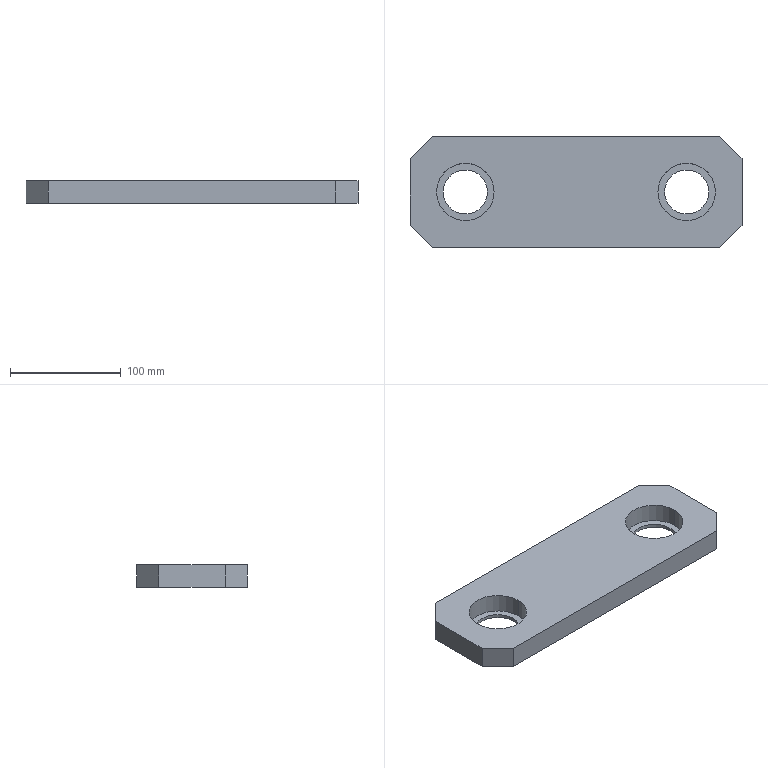Part | SolidWorks | features BaseBody 1 | 1 solid | 20 faces | box 300 x 100 x 20 mm | volume 504254 mm3 | plane 12 | cylinder 8 | commonest cylinder face diameters 40 x4 52 x4
STEP:
#1=CARTESIAN_POINT('',(198.047,1592.079,-399.));
#2=VERTEX_POINT('',#1);
#3=CARTESIAN_POINT('',(158.047,1592.079,-399.));
#4=VERTEX_POINT('',#3);
#5=CARTESIAN_POINT('',(178.047,1592.079,-399.));
#6=DIRECTION('',(0.,0.,-1.));
#7=DIRECTION('',(1.,0.,0.));
#8=AXIS2_PLACEMENT_3D('',#5,#6,#7);
#9=CIRCLE('',#8,20.);
#10=EDGE_CURVE('',#2,#4,#9,.T.);
#11=ORIENTED_EDGE('',*,*,#10,.T.);
#12=CARTESIAN_POINT('',(158.047,1592.079,-396.));
#13=VERTEX_POINT('',#12);
#14=CARTESIAN_POINT('',(158.047,1592.079,-455.569));
#15=DIRECTION('',(0.,0.,1.));
#16=VECTOR('',#15,1000.);
#17=LINE('',#14,#16);
#18=EDGE_CURVE('',#4,#13,#17,.T.);
#19=ORIENTED_EDGE('',*,*,#18,.T.);
#20=CARTESIAN_POINT('',(198.047,1592.079,-396.));
#21=VERTEX_POINT('',#20);
#22=CARTESIAN_POINT('',(178.047,1592.079,-396.));
#23=DIRECTION('',(0.,0.,-1.));
#24=DIRECTION('',(1.,0.,0.));
#25=AXIS2_PLACEMENT_3D('',#22,#23,#24);
#26=CIRCLE('',#25,20.);
#27=EDGE_CURVE('',#21,#13,#26,.T.);
#28=ORIENTED_EDGE('',*,*,#27,.F.);
#29=CARTESIAN_POINT('',(198.047,1592.079,-455.569));
#30=DIRECTION('',(0.,0.,1.));
#31=VECTOR('',#30,1000.);
#32=LINE('',#29,#31);
#33=EDGE_CURVE('',#2,#21,#32,.T.);
#34=ORIENTED_EDGE('',*,*,#33,.F.);
#35=EDGE_LOOP('',(#11,#19,#28,#34));
#36=FACE_OUTER_BOUND('',#35,.T.);
#37=CARTESIAN_POINT('',(178.047,1592.079,-455.569));
#38=DIRECTION('',(0.,0.,1.));
#39=DIRECTION('',(1.,0.,0.));
#40=AXIS2_PLACEMENT_3D('',#37,#38,#39);
#41=CYLINDRICAL_SURFACE('',#40,20.);
#42=ADVANCED_FACE('',(#36),#41,.F.);
#43=CARTESIAN_POINT('',(-1.953,1592.079,-399.));
#44=VERTEX_POINT('',#43);
#45=CARTESIAN_POINT('',(-41.953,1592.079,-399.));
#46=VERTEX_POINT('',#45);
#47=CARTESIAN_POINT('',(-21.953,1592.079,-399.));
#48=DIRECTION('',(0.,0.,-1.));
#49=DIRECTION('',(1.,0.,0.));
#50=AXIS2_PLACEMENT_3D('',#47,#48,#49);
#51=CIRCLE('',#50,20.);
#52=EDGE_CURVE('',#44,#46,#51,.T.);
#53=ORIENTED_EDGE('',*,*,#52,.T.);
#54=CARTESIAN_POINT('',(-41.953,1592.079,-396.));
#55=VERTEX_POINT('',#54);
#56=CARTESIAN_POINT('',(-41.953,1592.079,-455.569));
#57=DIRECTION('',(0.,0.,1.));
#58=VECTOR('',#57,1000.);
#59=LINE('',#56,#58);
#60=EDGE_CURVE('',#46,#55,#59,.T.);
#61=ORIENTED_EDGE('',*,*,#60,.T.);
#62=CARTESIAN_POINT('',(-1.953,1592.079,-396.));
#63=VERTEX_POINT('',#62);
#64=CARTESIAN_POINT('',(-21.953,1592.079,-396.));
#65=DIRECTION('',(0.,0.,-1.));
#66=DIRECTION('',(1.,0.,0.));
#67=AXIS2_PLACEMENT_3D('',#64,#65,#66);
#68=CIRCLE('',#67,20.);
#69=EDGE_CURVE('',#63,#55,#68,.T.);
#70=ORIENTED_EDGE('',*,*,#69,.F.);
#71=CARTESIAN_POINT('',(-1.953,1592.079,-455.569));
#72=DIRECTION('',(0.,0.,1.));
#73=VECTOR('',#72,1000.);
#74=LINE('',#71,#73);
#75=EDGE_CURVE('',#44,#63,#74,.T.);
#76=ORIENTED_EDGE('',*,*,#75,.F.);
#77=EDGE_LOOP('',(#53,#61,#70,#76));
#78=FACE_OUTER_BOUND('',#77,.T.);
#79=CARTESIAN_POINT('',(-21.953,1592.079,-455.569));
#80=DIRECTION('',(0.,0.,1.));
#81=DIRECTION('',(1.,0.,0.));
#82=AXIS2_PLACEMENT_3D('',#79,#80,#81);
#83=CYLINDRICAL_SURFACE('',#82,20.);
#84=ADVANCED_FACE('',(#78),#83,.F.);
#85=CARTESIAN_POINT('',(204.047,1592.079,-396.));
#86=VERTEX_POINT('',#85);
#87=CARTESIAN_POINT('',(152.047,1592.079,-396.));
#88=VERTEX_POINT('',#87);
#89=CARTESIAN_POINT('',(178.047,1592.079,-396.));
#90=DIRECTION('',(0.,0.,-1.));
#91=DIRECTION('',(1.,0.,0.));
#92=AXIS2_PLACEMENT_3D('',#89,#90,#91);
#93=CIRCLE('',#92,26.);
#94=EDGE_CURVE('',#86,#88,#93,.T.);
#95=ORIENTED_EDGE('',*,*,#94,.T.);
#96=CARTESIAN_POINT('',(152.047,1592.079,-379.));
#97=VERTEX_POINT('',#96);
#98=CARTESIAN_POINT('',(152.047,1592.079,-396.));
#99=DIRECTION('',(0.,0.,1.));
#100=VECTOR('',#99,1000.);
#101=LINE('',#98,#100);
#102=EDGE_CURVE('',#88,#97,#101,.T.);
#103=ORIENTED_EDGE('',*,*,#102,.T.);
#104=CARTESIAN_POINT('',(204.047,1592.079,-379.));
#105=VERTEX_POINT('',#104);
#106=CARTESIAN_POINT('',(178.047,1592.079,-379.));
#107=DIRECTION('',(0.,0.,-1.));
#108=DIRECTION('',(1.,0.,0.));
#109=AXIS2_PLACEMENT_3D('',#106,#107,#108);
#110=CIRCLE('',#109,26.);
#111=EDGE_CURVE('',#105,#97,#110,.T.);
#112=ORIENTED_EDGE('',*,*,#111,.F.);
#113=CARTESIAN_POINT('',(204.047,1592.079,-396.));
#114=DIRECTION('',(0.,0.,1.));
#115=VECTOR('',#114,1000.);
#116=LINE('',#113,#115);
#117=EDGE_CURVE('',#86,#105,#116,.T.);
#118=ORIENTED_EDGE('',*,*,#117,.F.);
#119=EDGE_LOOP('',(#95,#103,#112,#118));
#120=FACE_OUTER_BOUND('',#119,.T.);
#121=CARTESIAN_POINT('',(178.047,1592.079,-396.));
#122=DIRECTION('',(0.,0.,1.));
#123=DIRECTION('',(1.,0.,0.));
#124=AXIS2_PLACEMENT_3D('',#121,#122,#123);
#125=CYLINDRICAL_SURFACE('',#124,26.);
#126=ADVANCED_FACE('',(#120),#125,.F.);
#127=CARTESIAN_POINT('',(-47.953,1592.079,-396.));
#128=VERTEX_POINT('',#127);
#129=CARTESIAN_POINT('',(4.047,1592.079,-396.));
#130=VERTEX_POINT('',#129);
#131=CARTESIAN_POINT('',(-21.953,1592.079,-396.));
#132=DIRECTION('',(0.,0.,1.));
#133=DIRECTION('',(1.,0.,0.));
#134=AXIS2_PLACEMENT_3D('',#131,#132,#133);
#135=CIRCLE('',#134,26.);
#136=EDGE_CURVE('',#128,#130,#135,.T.);
#137=ORIENTED_EDGE('',*,*,#136,.F.);
#138=CARTESIAN_POINT('',(-47.953,1592.079,-379.));
#139=VERTEX_POINT('',#138);
#140=CARTESIAN_POINT('',(-47.953,1592.079,-396.));
#141=DIRECTION('',(0.,0.,1.));
#142=VECTOR('',#141,1000.);
#143=LINE('',#140,#142);
#144=EDGE_CURVE('',#128,#139,#143,.T.);
#145=ORIENTED_EDGE('',*,*,#144,.T.);
#146=CARTESIAN_POINT('',(4.047,1592.079,-379.));
#147=VERTEX_POINT('',#146);
#148=CARTESIAN_POINT('',(-21.953,1592.079,-379.));
#149=DIRECTION('',(0.,0.,-1.));
#150=DIRECTION('',(1.,0.,0.));
#151=AXIS2_PLACEMENT_3D('',#148,#149,#150);
#152=CIRCLE('',#151,26.);
#153=EDGE_CURVE('',#147,#139,#152,.T.);
#154=ORIENTED_EDGE('',*,*,#153,.F.);
#155=CARTESIAN_POINT('',(4.047,1592.079,-396.));
#156=DIRECTION('',(0.,0.,1.));
#157=VECTOR('',#156,1000.);
#158=LINE('',#155,#157);
#159=EDGE_CURVE('',#130,#147,#158,.T.);
#160=ORIENTED_EDGE('',*,*,#159,.F.);
#161=EDGE_LOOP('',(#137,#145,#154,#160));
#162=FACE_OUTER_BOUND('',#161,.T.);
#163=CARTESIAN_POINT('',(-21.953,1592.079,-396.));
#164=DIRECTION('',(0.,0.,1.));
#165=DIRECTION('',(1.,0.,0.));
#166=AXIS2_PLACEMENT_3D('',#163,#164,#165);
#167=CYLINDRICAL_SURFACE('',#166,26.);
#168=ADVANCED_FACE('',(#162),#167,.F.);
#169=ORIENTED_EDGE('',*,*,#10,.F.);
#170=CARTESIAN_POINT('',(178.047,1592.079,-399.));
#171=DIRECTION('',(0.,0.,-1.));
#172=DIRECTION('',(1.,0.,0.));
#173=AXIS2_PLACEMENT_3D('',#170,#171,#172);
#174=CIRCLE('',#173,20.);
#175=EDGE_CURVE('',#4,#2,#174,.T.);
#176=ORIENTED_EDGE('',*,*,#175,.F.);
#177=EDGE_LOOP('',(#169,#176));
#178=FACE_BOUND('',#177,.T.);
#179=ORIENTED_EDGE('',*,*,#52,.F.);
#180=CARTESIAN_POINT('',(-21.953,1592.079,-399.));
#181=DIRECTION('',(0.,0.,-1.));
#182=DIRECTION('',(1.,0.,0.));
#183=AXIS2_PLACEMENT_3D('',#180,#181,#182);
#184=CIRCLE('',#183,20.);
#185=EDGE_CURVE('',#46,#44,#184,.T.);
#186=ORIENTED_EDGE('',*,*,#185,.F.);
#187=EDGE_LOOP('',(#179,#186));
#188=FACE_BOUND('',#187,.T.);
#189=CARTESIAN_POINT('',(228.047,1562.079,-399.));
#190=VERTEX_POINT('',#189);
#191=CARTESIAN_POINT('',(228.047,1622.079,-399.));
#192=VERTEX_POINT('',#191);
#193=CARTESIAN_POINT('',(228.047,1542.079,-399.));
#194=DIRECTION('',(0.,1.,0.));
#195=VECTOR('',#194,1000.);
#196=LINE('',#193,#195);
#197=EDGE_CURVE('',#190,#192,#196,.T.);
#198=ORIENTED_EDGE('',*,*,#197,.F.);
#199=CARTESIAN_POINT('',(208.047,1542.079,-399.));
#200=VERTEX_POINT('',#199);
#201=CARTESIAN_POINT('',(208.047,1542.079,-399.));
#202=DIRECTION('',(0.7071,0.7071,0.));
#203=VECTOR('',#202,1000.);
#204=LINE('',#201,#203);
#205=EDGE_CURVE('',#200,#190,#204,.T.);
#206=ORIENTED_EDGE('',*,*,#205,.F.);
#207=CARTESIAN_POINT('',(-51.953,1542.079,-399.));
#208=VERTEX_POINT('',#207);
#209=CARTESIAN_POINT('',(-71.953,1542.079,-399.));
#210=DIRECTION('',(1.,0.,0.));
#211=VECTOR('',#210,1000.);
#212=LINE('',#209,#211);
#213=EDGE_CURVE('',#208,#200,#212,.T.);
#214=ORIENTED_EDGE('',*,*,#213,.F.);
#215=CARTESIAN_POINT('',(-71.953,1562.079,-399.));
#216=VERTEX_POINT('',#215);
#217=CARTESIAN_POINT('',(-71.953,1562.079,-399.));
#218=DIRECTION('',(0.7071,-0.7071,0.));
#219=VECTOR('',#218,1000.);
#220=LINE('',#217,#219);
#221=EDGE_CURVE('',#216,#208,#220,.T.);
#222=ORIENTED_EDGE('',*,*,#221,.F.);
#223=CARTESIAN_POINT('',(-71.953,1622.079,-399.));
#224=VERTEX_POINT('',#223);
#225=CARTESIAN_POINT('',(-71.953,1542.079,-399.));
#226=DIRECTION('',(0.,-1.,0.));
#227=VECTOR('',#226,1000.);
#228=LINE('',#225,#227);
#229=EDGE_CURVE('',#224,#216,#228,.T.);
#230=ORIENTED_EDGE('',*,*,#229,.F.);
#231=CARTESIAN_POINT('',(-51.953,1642.079,-399.));
#232=VERTEX_POINT('',#231);
#233=CARTESIAN_POINT('',(-51.953,1642.079,-399.));
#234=DIRECTION('',(-0.7071,-0.7071,0.));
#235=VECTOR('',#234,1000.);
#236=LINE('',#233,#235);
#237=EDGE_CURVE('',#232,#224,#236,.T.);
#238=ORIENTED_EDGE('',*,*,#237,.F.);
#239=CARTESIAN_POINT('',(208.047,1642.079,-399.));
#240=VERTEX_POINT('',#239);
#241=CARTESIAN_POINT('',(-71.953,1642.079,-399.));
#242=DIRECTION('',(-1.,0.,0.));
#243=VECTOR('',#242,1000.);
#244=LINE('',#241,#243);
#245=EDGE_CURVE('',#240,#232,#244,.T.);
#246=ORIENTED_EDGE('',*,*,#245,.F.);
#247=CARTESIAN_POINT('',(228.047,1622.079,-399.));
#248=DIRECTION('',(-0.7071,0.7071,0.));
#249=VECTOR('',#248,1000.);
#250=LINE('',#247,#249);
#251=EDGE_CURVE('',#192,#240,#250,.T.);
#252=ORIENTED_EDGE('',*,*,#251,.F.);
#253=EDGE_LOOP('',(#198,#206,#214,#222,#230,#238,#246,#252));
#254=FACE_OUTER_BOUND('',#253,.T.);
#255=CARTESIAN_POINT('',(-71.953,1542.079,-399.));
#256=DIRECTION('',(0.,0.,1.));
#257=DIRECTION('',(1.,0.,0.));
#258=AXIS2_PLACEMENT_3D('',#255,#256,#257);
#259=PLANE('',#258);
#260=ADVANCED_FACE('',(#178,#188,#254),#259,.F.);
#261=ORIENTED_EDGE('',*,*,#18,.F.);
#262=ORIENTED_EDGE('',*,*,#175,.T.);
#263=ORIENTED_EDGE('',*,*,#33,.T.);
#264=CARTESIAN_POINT('',(178.047,1592.079,-396.));
#265=DIRECTION('',(0.,0.,-1.));
#266=DIRECTION('',(1.,0.,0.));
#267=AXIS2_PLACEMENT_3D('',#264,#265,#266);
#268=CIRCLE('',#267,20.);
#269=EDGE_CURVE('',#13,#21,#268,.T.);
#270=ORIENTED_EDGE('',*,*,#269,.F.);
#271=EDGE_LOOP('',(#261,#262,#263,#270));
#272=FACE_OUTER_BOUND('',#271,.T.);
#273=CARTESIAN_POINT('',(178.047,1592.079,-455.569));
#274=DIRECTION('',(0.,0.,1.));
#275=DIRECTION('',(1.,0.,0.));
#276=AXIS2_PLACEMENT_3D('',#273,#274,#275);
#277=CYLINDRICAL_SURFACE('',#276,20.);
#278=ADVANCED_FACE('',(#272),#277,.F.);
#279=ORIENTED_EDGE('',*,*,#60,.F.);
#280=ORIENTED_EDGE('',*,*,#185,.T.);
#281=ORIENTED_EDGE('',*,*,#75,.T.);
#282=CARTESIAN_POINT('',(-21.953,1592.079,-396.));
#283=DIRECTION('',(0.,0.,-1.));
#284=DIRECTION('',(1.,0.,0.));
#285=AXIS2_PLACEMENT_3D('',#282,#283,#284);
#286=CIRCLE('',#285,20.);
#287=EDGE_CURVE('',#55,#63,#286,.T.);
#288=ORIENTED_EDGE('',*,*,#287,.F.);
#289=EDGE_LOOP('',(#279,#280,#281,#288));
#290=FACE_OUTER_BOUND('',#289,.T.);
#291=CARTESIAN_POINT('',(-21.953,1592.079,-455.569));
#292=DIRECTION('',(0.,0.,1.));
#293=DIRECTION('',(1.,0.,0.));
#294=AXIS2_PLACEMENT_3D('',#291,#292,#293);
#295=CYLINDRICAL_SURFACE('',#294,20.);
#296=ADVANCED_FACE('',(#290),#295,.F.);
#297=ORIENTED_EDGE('',*,*,#251,.T.);
#298=CARTESIAN_POINT('',(208.047,1642.079,-379.));
#299=VERTEX_POINT('',#298);
#300=CARTESIAN_POINT('',(208.047,1642.079,-379.));
#301=DIRECTION('',(0.,0.,-1.));
#302=VECTOR('',#301,1000.);
#303=LINE('',#300,#302);
#304=EDGE_CURVE('',#299,#240,#303,.T.);
#305=ORIENTED_EDGE('',*,*,#304,.F.);
#306=CARTESIAN_POINT('',(228.047,1622.079,-379.));
#307=VERTEX_POINT('',#306);
#308=CARTESIAN_POINT('',(208.047,1642.079,-379.));
#309=DIRECTION('',(-0.7071,0.7071,0.));
#310=VECTOR('',#309,1000.);
#311=LINE('',#308,#310);
#312=EDGE_CURVE('',#307,#299,#311,.T.);
#313=ORIENTED_EDGE('',*,*,#312,.F.);
#314=CARTESIAN_POINT('',(228.047,1622.079,-379.));
#315=DIRECTION('',(0.,0.,1.));
#316=VECTOR('',#315,1000.);
#317=LINE('',#314,#316);
#318=EDGE_CURVE('',#192,#307,#317,.T.);
#319=ORIENTED_EDGE('',*,*,#318,.F.);
#320=EDGE_LOOP('',(#297,#305,#313,#319));
#321=FACE_OUTER_BOUND('',#320,.T.);
#322=CARTESIAN_POINT('',(208.047,1642.079,-379.));
#323=DIRECTION('',(-0.7071,-0.7071,0.));
#324=DIRECTION('',(0.7071,-0.7071,0.));
#325=AXIS2_PLACEMENT_3D('',#322,#323,#324);
#326=PLANE('',#325);
#327=ADVANCED_FACE('',(#321),#326,.F.);
#328=CARTESIAN_POINT('',(228.047,1562.079,-379.));
#329=VERTEX_POINT('',#328);
#330=CARTESIAN_POINT('',(228.047,1642.079,-379.));
#331=DIRECTION('',(0.,1.,0.));
#332=VECTOR('',#331,1000.);
#333=LINE('',#330,#332);
#334=EDGE_CURVE('',#329,#307,#333,.T.);
#335=ORIENTED_EDGE('',*,*,#334,.F.);
#336=CARTESIAN_POINT('',(228.047,1562.079,-379.));
#337=DIRECTION('',(0.,0.,1.));
#338=VECTOR('',#337,1000.);
#339=LINE('',#336,#338);
#340=EDGE_CURVE('',#190,#329,#339,.T.);
#341=ORIENTED_EDGE('',*,*,#340,.F.);
#342=ORIENTED_EDGE('',*,*,#197,.T.);
#343=ORIENTED_EDGE('',*,*,#318,.T.);
#344=EDGE_LOOP('',(#335,#341,#342,#343));
#345=FACE_OUTER_BOUND('',#344,.T.);
#346=CARTESIAN_POINT('',(228.047,1642.079,-379.));
#347=DIRECTION('',(-1.,0.,0.));
#348=DIRECTION('',(0.,0.,1.));
#349=AXIS2_PLACEMENT_3D('',#346,#347,#348);
#350=PLANE('',#349);
#351=ADVANCED_FACE('',(#345),#350,.F.);
#352=ORIENTED_EDGE('',*,*,#205,.T.);
#353=ORIENTED_EDGE('',*,*,#340,.T.);
#354=CARTESIAN_POINT('',(208.047,1542.079,-379.));
#355=VERTEX_POINT('',#354);
#356=CARTESIAN_POINT('',(228.047,1562.079,-379.));
#357=DIRECTION('',(0.7071,0.7071,0.));
#358=VECTOR('',#357,1000.);
#359=LINE('',#356,#358);
#360=EDGE_CURVE('',#355,#329,#359,.T.);
#361=ORIENTED_EDGE('',*,*,#360,.F.);
#362=CARTESIAN_POINT('',(208.047,1542.079,-379.));
#363=DIRECTION('',(0.,0.,1.));
#364=VECTOR('',#363,1000.);
#365=LINE('',#362,#364);
#366=EDGE_CURVE('',#200,#355,#365,.T.);
#367=ORIENTED_EDGE('',*,*,#366,.F.);
#368=EDGE_LOOP('',(#352,#353,#361,#367));
#369=FACE_OUTER_BOUND('',#368,.T.);
#370=CARTESIAN_POINT('',(228.047,1562.079,-379.));
#371=DIRECTION('',(-0.7071,0.7071,0.));
#372=DIRECTION('',(-0.7071,-0.7071,0.));
#373=AXIS2_PLACEMENT_3D('',#370,#371,#372);
#374=PLANE('',#373);
#375=ADVANCED_FACE('',(#369),#374,.F.);
#376=CARTESIAN_POINT('',(-51.953,1542.079,-379.));
#377=VERTEX_POINT('',#376);
#378=CARTESIAN_POINT('',(-71.953,1542.079,-379.));
#379=DIRECTION('',(1.,0.,0.));
#380=VECTOR('',#379,1000.);
#381=LINE('',#378,#380);
#382=EDGE_CURVE('',#377,#355,#381,.T.);
#383=ORIENTED_EDGE('',*,*,#382,.F.);
#384=CARTESIAN_POINT('',(-51.953,1542.079,-379.));
#385=DIRECTION('',(0.,0.,1.));
#386=VECTOR('',#385,1000.);
#387=LINE('',#384,#386);
#388=EDGE_CURVE('',#208,#377,#387,.T.);
#389=ORIENTED_EDGE('',*,*,#388,.F.);
#390=ORIENTED_EDGE('',*,*,#213,.T.);
#391=ORIENTED_EDGE('',*,*,#366,.T.);
#392=EDGE_LOOP('',(#383,#389,#390,#391));
#393=FACE_OUTER_BOUND('',#392,.T.);
#394=CARTESIAN_POINT('',(-71.953,1542.079,-379.));
#395=DIRECTION('',(0.,1.,0.));
#396=DIRECTION('',(0.,0.,1.));
#397=AXIS2_PLACEMENT_3D('',#394,#395,#396);
#398=PLANE('',#397);
#399=ADVANCED_FACE('',(#393),#398,.F.);
#400=ORIENTED_EDGE('',*,*,#221,.T.);
#401=ORIENTED_EDGE('',*,*,#388,.T.);
#402=CARTESIAN_POINT('',(-71.953,1562.079,-379.));
#403=VERTEX_POINT('',#402);
#404=CARTESIAN_POINT('',(-51.953,1542.079,-379.));
#405=DIRECTION('',(0.7071,-0.7071,0.));
#406=VECTOR('',#405,1000.);
#407=LINE('',#404,#406);
#408=EDGE_CURVE('',#403,#377,#407,.T.);
#409=ORIENTED_EDGE('',*,*,#408,.F.);
#410=CARTESIAN_POINT('',(-71.953,1562.079,-379.));
#411=DIRECTION('',(0.,0.,1.));
#412=VECTOR('',#411,1000.);
#413=LINE('',#410,#412);
#414=EDGE_CURVE('',#216,#403,#413,.T.);
#415=ORIENTED_EDGE('',*,*,#414,.F.);
#416=EDGE_LOOP('',(#400,#401,#409,#415));
#417=FACE_OUTER_BOUND('',#416,.T.);
#418=CARTESIAN_POINT('',(-51.953,1542.079,-379.));
#419=DIRECTION('',(0.7071,0.7071,0.));
#420=DIRECTION('',(-0.7071,0.7071,0.));
#421=AXIS2_PLACEMENT_3D('',#418,#419,#420);
#422=PLANE('',#421);
#423=ADVANCED_FACE('',(#417),#422,.F.);
#424=ORIENTED_EDGE('',*,*,#229,.T.);
#425=ORIENTED_EDGE('',*,*,#414,.T.);
#426=CARTESIAN_POINT('',(-71.953,1622.079,-379.));
#427=VERTEX_POINT('',#426);
#428=CARTESIAN_POINT('',(-71.953,1642.079,-379.));
#429=DIRECTION('',(0.,-1.,0.));
#430=VECTOR('',#429,1000.);
#431=LINE('',#428,#430);
#432=EDGE_CURVE('',#427,#403,#431,.T.);
#433=ORIENTED_EDGE('',*,*,#432,.F.);
#434=CARTESIAN_POINT('',(-71.953,1622.079,-379.));
#435=DIRECTION('',(0.,0.,1.));
#436=VECTOR('',#435,1000.);
#437=LINE('',#434,#436);
#438=EDGE_CURVE('',#224,#427,#437,.T.);
#439=ORIENTED_EDGE('',*,*,#438,.F.);
#440=EDGE_LOOP('',(#424,#425,#433,#439));
#441=FACE_OUTER_BOUND('',#440,.T.);
#442=CARTESIAN_POINT('',(-71.953,1642.079,-379.));
#443=DIRECTION('',(1.,0.,0.));
#444=DIRECTION('',(0.,0.,-1.));
#445=AXIS2_PLACEMENT_3D('',#442,#443,#444);
#446=PLANE('',#445);
#447=ADVANCED_FACE('',(#441),#446,.F.);
#448=ORIENTED_EDGE('',*,*,#237,.T.);
#449=ORIENTED_EDGE('',*,*,#438,.T.);
#450=CARTESIAN_POINT('',(-51.953,1642.079,-379.));
#451=VERTEX_POINT('',#450);
#452=CARTESIAN_POINT('',(-71.953,1622.079,-379.));
#453=DIRECTION('',(-0.7071,-0.7071,0.));
#454=VECTOR('',#453,1000.);
#455=LINE('',#452,#454);
#456=EDGE_CURVE('',#451,#427,#455,.T.);
#457=ORIENTED_EDGE('',*,*,#456,.F.);
#458=CARTESIAN_POINT('',(-51.953,1642.079,-379.));
#459=DIRECTION('',(0.,0.,1.));
#460=VECTOR('',#459,1000.);
#461=LINE('',#458,#460);
#462=EDGE_CURVE('',#232,#451,#461,.T.);
#463=ORIENTED_EDGE('',*,*,#462,.F.);
#464=EDGE_LOOP('',(#448,#449,#457,#463));
#465=FACE_OUTER_BOUND('',#464,.T.);
#466=CARTESIAN_POINT('',(-71.953,1622.079,-379.));
#467=DIRECTION('',(0.7071,-0.7071,0.));
#468=DIRECTION('',(0.7071,0.7071,0.));
#469=AXIS2_PLACEMENT_3D('',#466,#467,#468);
#470=PLANE('',#469);
#471=ADVANCED_FACE('',(#465),#470,.F.);
#472=ORIENTED_EDGE('',*,*,#245,.T.);
#473=ORIENTED_EDGE('',*,*,#462,.T.);
#474=CARTESIAN_POINT('',(-71.953,1642.079,-379.));
#475=DIRECTION('',(-1.,0.,0.));
#476=VECTOR('',#475,1000.);
#477=LINE('',#474,#476);
#478=EDGE_CURVE('',#299,#451,#477,.T.);
#479=ORIENTED_EDGE('',*,*,#478,.F.);
#480=ORIENTED_EDGE('',*,*,#304,.T.);
#481=EDGE_LOOP('',(#472,#473,#479,#480));
#482=FACE_OUTER_BOUND('',#481,.T.);
#483=CARTESIAN_POINT('',(-71.953,1642.079,-379.));
#484=DIRECTION('',(0.,-1.,0.));
#485=DIRECTION('',(0.,0.,-1.));
#486=AXIS2_PLACEMENT_3D('',#483,#484,#485);
#487=PLANE('',#486);
#488=ADVANCED_FACE('',(#482),#487,.F.);
#489=ORIENTED_EDGE('',*,*,#27,.T.);
#490=ORIENTED_EDGE('',*,*,#269,.T.);
#491=EDGE_LOOP('',(#489,#490));
#492=FACE_BOUND('',#491,.T.);
#493=ORIENTED_EDGE('',*,*,#94,.F.);
#494=CARTESIAN_POINT('',(178.047,1592.079,-396.));
#495=DIRECTION('',(0.,0.,-1.));
#496=DIRECTION('',(1.,0.,0.));
#497=AXIS2_PLACEMENT_3D('',#494,#495,#496);
#498=CIRCLE('',#497,26.);
#499=EDGE_CURVE('',#88,#86,#498,.T.);
#500=ORIENTED_EDGE('',*,*,#499,.F.);
#501=EDGE_LOOP('',(#493,#500));
#502=FACE_OUTER_BOUND('',#501,.T.);
#503=CARTESIAN_POINT('',(178.047,1592.079,-396.));
#504=DIRECTION('',(0.,0.,-1.));
#505=DIRECTION('',(-1.,0.,0.));
#506=AXIS2_PLACEMENT_3D('',#503,#504,#505);
#507=PLANE('',#506);
#508=ADVANCED_FACE('',(#492,#502),#507,.F.);
#509=ORIENTED_EDGE('',*,*,#69,.T.);
#510=ORIENTED_EDGE('',*,*,#287,.T.);
#511=EDGE_LOOP('',(#509,#510));
#512=FACE_BOUND('',#511,.T.);
#513=CARTESIAN_POINT('',(-21.953,1592.079,-396.));
#514=DIRECTION('',(0.,0.,1.));
#515=DIRECTION('',(1.,0.,0.));
#516=AXIS2_PLACEMENT_3D('',#513,#514,#515);
#517=CIRCLE('',#516,26.);
#518=EDGE_CURVE('',#130,#128,#517,.T.);
#519=ORIENTED_EDGE('',*,*,#518,.T.);
#520=ORIENTED_EDGE('',*,*,#136,.T.);
#521=EDGE_LOOP('',(#519,#520));
#522=FACE_OUTER_BOUND('',#521,.T.);
#523=CARTESIAN_POINT('',(-21.953,1592.079,-396.));
#524=DIRECTION('',(0.,0.,1.));
#525=DIRECTION('',(1.,0.,0.));
#526=AXIS2_PLACEMENT_3D('',#523,#524,#525);
#527=PLANE('',#526);
#528=ADVANCED_FACE('',(#512,#522),#527,.T.);
#529=ORIENTED_EDGE('',*,*,#111,.T.);
#530=CARTESIAN_POINT('',(178.047,1592.079,-379.));
#531=DIRECTION('',(0.,0.,-1.));
#532=DIRECTION('',(1.,0.,0.));
#533=AXIS2_PLACEMENT_3D('',#530,#531,#532);
#534=CIRCLE('',#533,26.);
#535=EDGE_CURVE('',#97,#105,#534,.T.);
#536=ORIENTED_EDGE('',*,*,#535,.T.);
#537=EDGE_LOOP('',(#529,#536));
#538=FACE_BOUND('',#537,.T.);
#539=ORIENTED_EDGE('',*,*,#153,.T.);
#540=CARTESIAN_POINT('',(-21.953,1592.079,-379.));
#541=DIRECTION('',(0.,0.,-1.));
#542=DIRECTION('',(1.,0.,0.));
#543=AXIS2_PLACEMENT_3D('',#540,#541,#542);
#544=CIRCLE('',#543,26.);
#545=EDGE_CURVE('',#139,#147,#544,.T.);
#546=ORIENTED_EDGE('',*,*,#545,.T.);
#547=EDGE_LOOP('',(#539,#546));
#548=FACE_BOUND('',#547,.T.);
#549=ORIENTED_EDGE('',*,*,#360,.T.);
#550=ORIENTED_EDGE('',*,*,#334,.T.);
#551=ORIENTED_EDGE('',*,*,#312,.T.);
#552=ORIENTED_EDGE('',*,*,#478,.T.);
#553=ORIENTED_EDGE('',*,*,#456,.T.);
#554=ORIENTED_EDGE('',*,*,#432,.T.);
#555=ORIENTED_EDGE('',*,*,#408,.T.);
#556=ORIENTED_EDGE('',*,*,#382,.T.);
#557=EDGE_LOOP('',(#549,#550,#551,#552,#553,#554,#555,#556));
#558=FACE_OUTER_BOUND('',#557,.T.);
#559=CARTESIAN_POINT('',(-71.953,1542.079,-379.));
#560=DIRECTION('',(0.,0.,1.));
#561=DIRECTION('',(1.,0.,0.));
#562=AXIS2_PLACEMENT_3D('',#559,#560,#561);
#563=PLANE('',#562);
#564=ADVANCED_FACE('',(#538,#548,#558),#563,.T.);
#565=ORIENTED_EDGE('',*,*,#102,.F.);
#566=ORIENTED_EDGE('',*,*,#499,.T.);
#567=ORIENTED_EDGE('',*,*,#117,.T.);
#568=ORIENTED_EDGE('',*,*,#535,.F.);
#569=EDGE_LOOP('',(#565,#566,#567,#568));
#570=FACE_OUTER_BOUND('',#569,.T.);
#571=CARTESIAN_POINT('',(178.047,1592.079,-396.));
#572=DIRECTION('',(0.,0.,1.));
#573=DIRECTION('',(1.,0.,0.));
#574=AXIS2_PLACEMENT_3D('',#571,#572,#573);
#575=CYLINDRICAL_SURFACE('',#574,26.);
#576=ADVANCED_FACE('',(#570),#575,.F.);
#577=ORIENTED_EDGE('',*,*,#144,.F.);
#578=ORIENTED_EDGE('',*,*,#518,.F.);
#579=ORIENTED_EDGE('',*,*,#159,.T.);
#580=ORIENTED_EDGE('',*,*,#545,.F.);
#581=EDGE_LOOP('',(#577,#578,#579,#580));
#582=FACE_OUTER_BOUND('',#581,.T.);
#583=CARTESIAN_POINT('',(-21.953,1592.079,-396.));
#584=DIRECTION('',(0.,0.,1.));
#585=DIRECTION('',(1.,0.,0.));
#586=AXIS2_PLACEMENT_3D('',#583,#584,#585);
#587=CYLINDRICAL_SURFACE('',#586,26.);
#588=ADVANCED_FACE('',(#582),#587,.F.);
#589=CLOSED_SHELL('',(#42,#84,#126,#168,#260,#278,#296,#327,#351,#375,#399,#423,#447,#471,#488,#508,#528,#564,#576,#588));
#590=MANIFOLD_SOLID_BREP('',#589);
#591=CARTESIAN_POINT('',(0.,0.,0.));
#592=DIRECTION('',(0.,0.,1.));
#593=DIRECTION('',(1.,0.,0.));
#594=AXIS2_PLACEMENT_3D('',#591,#592,#593);
#595=(LENGTH_UNIT()NAMED_UNIT(*)SI_UNIT(.MILLI.,.METRE.));
#596=UNCERTAINTY_MEASURE_WITH_UNIT(LENGTH_MEASURE(0.00001),#595,'','');
#597=(NAMED_UNIT(*)PLANE_ANGLE_UNIT()SI_UNIT($,.RADIAN.));
#598=(NAMED_UNIT(*)SI_UNIT($,.STERADIAN.)SOLID_ANGLE_UNIT());
#599=(GEOMETRIC_REPRESENTATION_CONTEXT(3)GLOBAL_UNCERTAINTY_ASSIGNED_CONTEXT((#596))GLOBAL_UNIT_ASSIGNED_CONTEXT((#595,#597,#598))REPRESENTATION_CONTEXT('',''));
#600=ADVANCED_BREP_SHAPE_REPRESENTATION('',(#590,#594),#599);